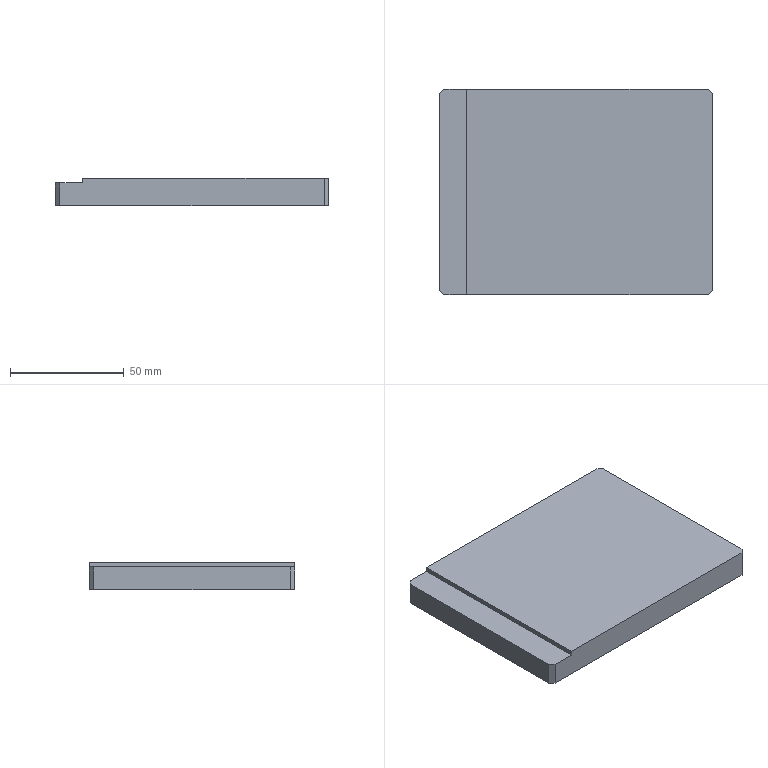Part | STEP file | 001-005-Shaft threading fixture base plate | 1 solid | 12 faces | box 120 x 90 x 12 mm | volume 127352 mm3 | plane 12
STEP:
#1=CARTESIAN_POINT('',(0.,0.,0.));
#2=DIRECTION('',(0.,0.,1.));
#3=DIRECTION('',(1.,0.,0.));
#4=AXIS2_PLACEMENT_3D('',#1,#2,#3);
#5=CARTESIAN_POINT('',(60.,-43.,12.));
#6=VERTEX_POINT('',#5);
#7=CARTESIAN_POINT('',(60.,43.,12.));
#8=VERTEX_POINT('',#7);
#9=CARTESIAN_POINT('',(60.,45.,12.));
#10=DIRECTION('',(0.,1.,0.));
#11=VECTOR('',#10,1.);
#12=LINE('',#9,#11);
#13=CARTESIAN_POINT('',(60.,45.,12.));
#14=DIRECTION('',(-1.,0.,0.));
#15=DIRECTION('',(0.,-1.,0.));
#16=AXIS2_PLACEMENT_3D('',#13,#14,#15);
#17=PLANE('',#16);
#18=CARTESIAN_POINT('',(0.,0.));
#19=DIRECTION('',(-1.,0.));
#20=VECTOR('',#19,1.);
#21=LINE('',#18,#20);
#22=(GEOMETRIC_REPRESENTATION_CONTEXT(2)PARAMETRIC_REPRESENTATION_CONTEXT()REPRESENTATION_CONTEXT('',''));
#23=DEFINITIONAL_REPRESENTATION('',(#21),#22);
#24=PCURVE('',#17,#23);
#25=CARTESIAN_POINT('',(0.,0.,12.));
#26=DIRECTION('',(0.,0.,1.));
#27=DIRECTION('',(1.,0.,0.));
#28=AXIS2_PLACEMENT_3D('',#25,#26,#27);
#29=PLANE('',#28);
#30=CARTESIAN_POINT('',(60.,45.));
#31=DIRECTION('',(0.,1.));
#32=VECTOR('',#31,1.);
#33=LINE('',#30,#32);
#34=(GEOMETRIC_REPRESENTATION_CONTEXT(2)PARAMETRIC_REPRESENTATION_CONTEXT()REPRESENTATION_CONTEXT('',''));
#35=DEFINITIONAL_REPRESENTATION('',(#33),#34);
#36=PCURVE('',#29,#35);
#37=SURFACE_CURVE('',#12,(#24,#36),.PCURVE_S1.);
#38=EDGE_CURVE('',#6,#8,#37,.T.);
#39=ORIENTED_EDGE('',*,*,#38,.F.);
#40=CARTESIAN_POINT('',(60.,-43.,0.));
#41=VERTEX_POINT('',#40);
#42=CARTESIAN_POINT('',(60.,-43.,12.));
#43=DIRECTION('',(0.,0.,-1.));
#44=VECTOR('',#43,1.);
#45=LINE('',#42,#44);
#46=CARTESIAN_POINT('',(88.,0.));
#47=DIRECTION('',(0.,-1.));
#48=VECTOR('',#47,1.);
#49=LINE('',#46,#48);
#50=(GEOMETRIC_REPRESENTATION_CONTEXT(2)PARAMETRIC_REPRESENTATION_CONTEXT()REPRESENTATION_CONTEXT('',''));
#51=DEFINITIONAL_REPRESENTATION('',(#49),#50);
#52=PCURVE('',#17,#51);
#53=CARTESIAN_POINT('',(60.,-43.,12.));
#54=DIRECTION('',(-0.7071,0.7071,0.));
#55=DIRECTION('',(0.,0.,-1.));
#56=AXIS2_PLACEMENT_3D('',#53,#54,#55);
#57=PLANE('',#56);
#58=CARTESIAN_POINT('',(0.,0.));
#59=DIRECTION('',(1.,0.));
#60=VECTOR('',#59,1.);
#61=LINE('',#58,#60);
#62=(GEOMETRIC_REPRESENTATION_CONTEXT(2)PARAMETRIC_REPRESENTATION_CONTEXT()REPRESENTATION_CONTEXT('',''));
#63=DEFINITIONAL_REPRESENTATION('',(#61),#62);
#64=PCURVE('',#57,#63);
#65=SURFACE_CURVE('',#45,(#52,#64),.PCURVE_S1.);
#66=EDGE_CURVE('',#6,#41,#65,.T.);
#67=ORIENTED_EDGE('',*,*,#66,.T.);
#68=CARTESIAN_POINT('',(60.,43.,0.));
#69=VERTEX_POINT('',#68);
#70=CARTESIAN_POINT('',(60.,45.,0.));
#71=DIRECTION('',(0.,1.,0.));
#72=VECTOR('',#71,1.);
#73=LINE('',#70,#72);
#74=CARTESIAN_POINT('',(0.,-12.));
#75=DIRECTION('',(-1.,0.));
#76=VECTOR('',#75,1.);
#77=LINE('',#74,#76);
#78=(GEOMETRIC_REPRESENTATION_CONTEXT(2)PARAMETRIC_REPRESENTATION_CONTEXT()REPRESENTATION_CONTEXT('',''));
#79=DEFINITIONAL_REPRESENTATION('',(#77),#78);
#80=PCURVE('',#17,#79);
#81=CARTESIAN_POINT('',(0.,0.,0.));
#82=DIRECTION('',(0.,0.,1.));
#83=DIRECTION('',(1.,0.,0.));
#84=AXIS2_PLACEMENT_3D('',#81,#82,#83);
#85=PLANE('',#84);
#86=CARTESIAN_POINT('',(60.,45.));
#87=DIRECTION('',(0.,1.));
#88=VECTOR('',#87,1.);
#89=LINE('',#86,#88);
#90=(GEOMETRIC_REPRESENTATION_CONTEXT(2)PARAMETRIC_REPRESENTATION_CONTEXT()REPRESENTATION_CONTEXT('',''));
#91=DEFINITIONAL_REPRESENTATION('',(#89),#90);
#92=PCURVE('',#85,#91);
#93=SURFACE_CURVE('',#73,(#80,#92),.PCURVE_S1.);
#94=EDGE_CURVE('',#41,#69,#93,.T.);
#95=ORIENTED_EDGE('',*,*,#94,.T.);
#96=CARTESIAN_POINT('',(60.,43.,12.));
#97=DIRECTION('',(0.,0.,1.));
#98=VECTOR('',#97,1.);
#99=LINE('',#96,#98);
#100=CARTESIAN_POINT('',(2.,0.));
#101=DIRECTION('',(0.,1.));
#102=VECTOR('',#101,1.);
#103=LINE('',#100,#102);
#104=(GEOMETRIC_REPRESENTATION_CONTEXT(2)PARAMETRIC_REPRESENTATION_CONTEXT()REPRESENTATION_CONTEXT('',''));
#105=DEFINITIONAL_REPRESENTATION('',(#103),#104);
#106=PCURVE('',#17,#105);
#107=CARTESIAN_POINT('',(58.,45.,12.));
#108=DIRECTION('',(-0.7071,-0.7071,0.));
#109=DIRECTION('',(0.,0.,-1.));
#110=AXIS2_PLACEMENT_3D('',#107,#108,#109);
#111=PLANE('',#110);
#112=CARTESIAN_POINT('',(0.,2.828));
#113=DIRECTION('',(-1.,0.));
#114=VECTOR('',#113,1.);
#115=LINE('',#112,#114);
#116=(GEOMETRIC_REPRESENTATION_CONTEXT(2)PARAMETRIC_REPRESENTATION_CONTEXT()REPRESENTATION_CONTEXT('',''));
#117=DEFINITIONAL_REPRESENTATION('',(#115),#116);
#118=PCURVE('',#111,#117);
#119=SURFACE_CURVE('',#99,(#106,#118),.PCURVE_S1.);
#120=EDGE_CURVE('',#69,#8,#119,.T.);
#121=ORIENTED_EDGE('',*,*,#120,.T.);
#122=EDGE_LOOP('',(#39,#67,#95,#121));
#123=FACE_BOUND('',#122,.T.);
#124=ADVANCED_FACE('',(#123),#17,.F.);
#125=CARTESIAN_POINT('',(-58.,45.,10.));
#126=VERTEX_POINT('',#125);
#127=CARTESIAN_POINT('',(-48.,45.,10.));
#128=VERTEX_POINT('',#127);
#129=CARTESIAN_POINT('',(-48.,45.,10.));
#130=DIRECTION('',(1.,0.,0.));
#131=VECTOR('',#130,1.);
#132=LINE('',#129,#131);
#133=CARTESIAN_POINT('',(-60.,45.,12.));
#134=DIRECTION('',(0.,-1.,0.));
#135=DIRECTION('',(0.,0.,-1.));
#136=AXIS2_PLACEMENT_3D('',#133,#134,#135);
#137=PLANE('',#136);
#138=CARTESIAN_POINT('',(2.,12.));
#139=DIRECTION('',(0.,1.));
#140=VECTOR('',#139,1.);
#141=LINE('',#138,#140);
#142=(GEOMETRIC_REPRESENTATION_CONTEXT(2)PARAMETRIC_REPRESENTATION_CONTEXT()REPRESENTATION_CONTEXT('',''));
#143=DEFINITIONAL_REPRESENTATION('',(#141),#142);
#144=PCURVE('',#137,#143);
#145=CARTESIAN_POINT('',(-48.,45.,10.));
#146=DIRECTION('',(0.,0.,-1.));
#147=DIRECTION('',(-1.,0.,0.));
#148=AXIS2_PLACEMENT_3D('',#145,#146,#147);
#149=PLANE('',#148);
#150=CARTESIAN_POINT('',(0.,0.));
#151=DIRECTION('',(-1.,0.));
#152=VECTOR('',#151,1.);
#153=LINE('',#150,#152);
#154=(GEOMETRIC_REPRESENTATION_CONTEXT(2)PARAMETRIC_REPRESENTATION_CONTEXT()REPRESENTATION_CONTEXT('',''));
#155=DEFINITIONAL_REPRESENTATION('',(#153),#154);
#156=PCURVE('',#149,#155);
#157=SURFACE_CURVE('',#132,(#144,#156),.PCURVE_S1.);
#158=EDGE_CURVE('',#126,#128,#157,.T.);
#159=ORIENTED_EDGE('',*,*,#158,.T.);
#160=CARTESIAN_POINT('',(-48.,45.,12.));
#161=VERTEX_POINT('',#160);
#162=CARTESIAN_POINT('',(-48.,45.,12.));
#163=DIRECTION('',(0.,0.,1.));
#164=VECTOR('',#163,1.);
#165=LINE('',#162,#164);
#166=CARTESIAN_POINT('',(0.,12.));
#167=DIRECTION('',(-1.,0.));
#168=VECTOR('',#167,1.);
#169=LINE('',#166,#168);
#170=(GEOMETRIC_REPRESENTATION_CONTEXT(2)PARAMETRIC_REPRESENTATION_CONTEXT()REPRESENTATION_CONTEXT('',''));
#171=DEFINITIONAL_REPRESENTATION('',(#169),#170);
#172=PCURVE('',#137,#171);
#173=CARTESIAN_POINT('',(-48.,45.,12.));
#174=DIRECTION('',(1.,0.,0.));
#175=DIRECTION('',(0.,1.,0.));
#176=AXIS2_PLACEMENT_3D('',#173,#174,#175);
#177=PLANE('',#176);
#178=CARTESIAN_POINT('',(0.,0.));
#179=DIRECTION('',(0.,1.));
#180=VECTOR('',#179,1.);
#181=LINE('',#178,#180);
#182=(GEOMETRIC_REPRESENTATION_CONTEXT(2)PARAMETRIC_REPRESENTATION_CONTEXT()REPRESENTATION_CONTEXT('',''));
#183=DEFINITIONAL_REPRESENTATION('',(#181),#182);
#184=PCURVE('',#177,#183);
#185=SURFACE_CURVE('',#165,(#172,#184),.PCURVE_S1.);
#186=EDGE_CURVE('',#128,#161,#185,.T.);
#187=ORIENTED_EDGE('',*,*,#186,.T.);
#188=CARTESIAN_POINT('',(58.,45.,12.));
#189=VERTEX_POINT('',#188);
#190=CARTESIAN_POINT('',(-60.,45.,12.));
#191=DIRECTION('',(-1.,0.,0.));
#192=VECTOR('',#191,1.);
#193=LINE('',#190,#192);
#194=CARTESIAN_POINT('',(0.,0.));
#195=DIRECTION('',(0.,-1.));
#196=VECTOR('',#195,1.);
#197=LINE('',#194,#196);
#198=(GEOMETRIC_REPRESENTATION_CONTEXT(2)PARAMETRIC_REPRESENTATION_CONTEXT()REPRESENTATION_CONTEXT('',''));
#199=DEFINITIONAL_REPRESENTATION('',(#197),#198);
#200=PCURVE('',#137,#199);
#201=CARTESIAN_POINT('',(-60.,45.));
#202=DIRECTION('',(-1.,0.));
#203=VECTOR('',#202,1.);
#204=LINE('',#201,#203);
#205=(GEOMETRIC_REPRESENTATION_CONTEXT(2)PARAMETRIC_REPRESENTATION_CONTEXT()REPRESENTATION_CONTEXT('',''));
#206=DEFINITIONAL_REPRESENTATION('',(#204),#205);
#207=PCURVE('',#29,#206);
#208=SURFACE_CURVE('',#193,(#200,#207),.PCURVE_S1.);
#209=EDGE_CURVE('',#189,#161,#208,.T.);
#210=ORIENTED_EDGE('',*,*,#209,.F.);
#211=CARTESIAN_POINT('',(58.,45.,0.));
#212=VERTEX_POINT('',#211);
#213=CARTESIAN_POINT('',(58.,45.,12.));
#214=DIRECTION('',(0.,0.,-1.));
#215=VECTOR('',#214,1.);
#216=LINE('',#213,#215);
#217=CARTESIAN_POINT('',(0.,118.));
#218=DIRECTION('',(1.,0.));
#219=VECTOR('',#218,1.);
#220=LINE('',#217,#219);
#221=(GEOMETRIC_REPRESENTATION_CONTEXT(2)PARAMETRIC_REPRESENTATION_CONTEXT()REPRESENTATION_CONTEXT('',''));
#222=DEFINITIONAL_REPRESENTATION('',(#220),#221);
#223=PCURVE('',#137,#222);
#224=CARTESIAN_POINT('',(0.,0.));
#225=DIRECTION('',(1.,0.));
#226=VECTOR('',#225,1.);
#227=LINE('',#224,#226);
#228=(GEOMETRIC_REPRESENTATION_CONTEXT(2)PARAMETRIC_REPRESENTATION_CONTEXT()REPRESENTATION_CONTEXT('',''));
#229=DEFINITIONAL_REPRESENTATION('',(#227),#228);
#230=PCURVE('',#111,#229);
#231=SURFACE_CURVE('',#216,(#223,#230),.PCURVE_S1.);
#232=EDGE_CURVE('',#189,#212,#231,.T.);
#233=ORIENTED_EDGE('',*,*,#232,.T.);
#234=CARTESIAN_POINT('',(-58.,45.,0.));
#235=VERTEX_POINT('',#234);
#236=CARTESIAN_POINT('',(-60.,45.,0.));
#237=DIRECTION('',(-1.,0.,0.));
#238=VECTOR('',#237,1.);
#239=LINE('',#236,#238);
#240=CARTESIAN_POINT('',(12.,0.));
#241=DIRECTION('',(0.,-1.));
#242=VECTOR('',#241,1.);
#243=LINE('',#240,#242);
#244=(GEOMETRIC_REPRESENTATION_CONTEXT(2)PARAMETRIC_REPRESENTATION_CONTEXT()REPRESENTATION_CONTEXT('',''));
#245=DEFINITIONAL_REPRESENTATION('',(#243),#244);
#246=PCURVE('',#137,#245);
#247=CARTESIAN_POINT('',(-60.,45.));
#248=DIRECTION('',(-1.,0.));
#249=VECTOR('',#248,1.);
#250=LINE('',#247,#249);
#251=(GEOMETRIC_REPRESENTATION_CONTEXT(2)PARAMETRIC_REPRESENTATION_CONTEXT()REPRESENTATION_CONTEXT('',''));
#252=DEFINITIONAL_REPRESENTATION('',(#250),#251);
#253=PCURVE('',#85,#252);
#254=SURFACE_CURVE('',#239,(#246,#253),.PCURVE_S1.);
#255=EDGE_CURVE('',#212,#235,#254,.T.);
#256=ORIENTED_EDGE('',*,*,#255,.T.);
#257=CARTESIAN_POINT('',(-58.,45.,12.));
#258=DIRECTION('',(0.,0.,1.));
#259=VECTOR('',#258,1.);
#260=LINE('',#257,#259);
#261=CARTESIAN_POINT('',(0.,2.));
#262=DIRECTION('',(-1.,0.));
#263=VECTOR('',#262,1.);
#264=LINE('',#261,#263);
#265=(GEOMETRIC_REPRESENTATION_CONTEXT(2)PARAMETRIC_REPRESENTATION_CONTEXT()REPRESENTATION_CONTEXT('',''));
#266=DEFINITIONAL_REPRESENTATION('',(#264),#265);
#267=PCURVE('',#137,#266);
#268=CARTESIAN_POINT('',(-60.,43.,12.));
#269=DIRECTION('',(0.7071,-0.7071,0.));
#270=DIRECTION('',(0.,0.,-1.));
#271=AXIS2_PLACEMENT_3D('',#268,#269,#270);
#272=PLANE('',#271);
#273=CARTESIAN_POINT('',(0.,2.828));
#274=DIRECTION('',(-1.,0.));
#275=VECTOR('',#274,1.);
#276=LINE('',#273,#275);
#277=(GEOMETRIC_REPRESENTATION_CONTEXT(2)PARAMETRIC_REPRESENTATION_CONTEXT()REPRESENTATION_CONTEXT('',''));
#278=DEFINITIONAL_REPRESENTATION('',(#276),#277);
#279=PCURVE('',#272,#278);
#280=SURFACE_CURVE('',#260,(#267,#279),.PCURVE_S1.);
#281=EDGE_CURVE('',#235,#126,#280,.T.);
#282=ORIENTED_EDGE('',*,*,#281,.T.);
#283=EDGE_LOOP('',(#159,#187,#210,#233,#256,#282));
#284=FACE_BOUND('',#283,.T.);
#285=ADVANCED_FACE('',(#284),#137,.F.);
#286=CARTESIAN_POINT('',(-60.,-43.,0.));
#287=VERTEX_POINT('',#286);
#288=CARTESIAN_POINT('',(-60.,-43.,10.));
#289=VERTEX_POINT('',#288);
#290=CARTESIAN_POINT('',(-60.,-43.,12.));
#291=DIRECTION('',(0.,0.,1.));
#292=VECTOR('',#291,1.);
#293=LINE('',#290,#292);
#294=CARTESIAN_POINT('',(-60.,45.,12.));
#295=DIRECTION('',(1.,0.,0.));
#296=DIRECTION('',(0.,1.,0.));
#297=AXIS2_PLACEMENT_3D('',#294,#295,#296);
#298=PLANE('',#297);
#299=CARTESIAN_POINT('',(-88.,0.));
#300=DIRECTION('',(0.,1.));
#301=VECTOR('',#300,1.);
#302=LINE('',#299,#301);
#303=(GEOMETRIC_REPRESENTATION_CONTEXT(2)PARAMETRIC_REPRESENTATION_CONTEXT()REPRESENTATION_CONTEXT('',''));
#304=DEFINITIONAL_REPRESENTATION('',(#302),#303);
#305=PCURVE('',#298,#304);
#306=CARTESIAN_POINT('',(-58.,-45.,12.));
#307=DIRECTION('',(0.7071,0.7071,0.));
#308=DIRECTION('',(0.,0.,-1.));
#309=AXIS2_PLACEMENT_3D('',#306,#307,#308);
#310=PLANE('',#309);
#311=CARTESIAN_POINT('',(0.,2.828));
#312=DIRECTION('',(-1.,0.));
#313=VECTOR('',#312,1.);
#314=LINE('',#311,#313);
#315=(GEOMETRIC_REPRESENTATION_CONTEXT(2)PARAMETRIC_REPRESENTATION_CONTEXT()REPRESENTATION_CONTEXT('',''));
#316=DEFINITIONAL_REPRESENTATION('',(#314),#315);
#317=PCURVE('',#310,#316);
#318=SURFACE_CURVE('',#293,(#305,#317),.PCURVE_S1.);
#319=EDGE_CURVE('',#287,#289,#318,.T.);
#320=ORIENTED_EDGE('',*,*,#319,.T.);
#321=CARTESIAN_POINT('',(-60.,43.,10.));
#322=VERTEX_POINT('',#321);
#323=CARTESIAN_POINT('',(-60.,45.,10.));
#324=DIRECTION('',(0.,-1.,0.));
#325=VECTOR('',#324,1.);
#326=LINE('',#323,#325);
#327=CARTESIAN_POINT('',(0.,-2.));
#328=DIRECTION('',(-1.,0.));
#329=VECTOR('',#328,1.);
#330=LINE('',#327,#329);
#331=(GEOMETRIC_REPRESENTATION_CONTEXT(2)PARAMETRIC_REPRESENTATION_CONTEXT()REPRESENTATION_CONTEXT('',''));
#332=DEFINITIONAL_REPRESENTATION('',(#330),#331);
#333=PCURVE('',#298,#332);
#334=CARTESIAN_POINT('',(12.,0.));
#335=DIRECTION('',(0.,-1.));
#336=VECTOR('',#335,1.);
#337=LINE('',#334,#336);
#338=(GEOMETRIC_REPRESENTATION_CONTEXT(2)PARAMETRIC_REPRESENTATION_CONTEXT()REPRESENTATION_CONTEXT('',''));
#339=DEFINITIONAL_REPRESENTATION('',(#337),#338);
#340=PCURVE('',#149,#339);
#341=SURFACE_CURVE('',#326,(#333,#340),.PCURVE_S1.);
#342=EDGE_CURVE('',#322,#289,#341,.T.);
#343=ORIENTED_EDGE('',*,*,#342,.F.);
#344=CARTESIAN_POINT('',(-60.,43.,0.));
#345=VERTEX_POINT('',#344);
#346=CARTESIAN_POINT('',(-60.,43.,12.));
#347=DIRECTION('',(0.,0.,-1.));
#348=VECTOR('',#347,1.);
#349=LINE('',#346,#348);
#350=CARTESIAN_POINT('',(-2.,0.));
#351=DIRECTION('',(0.,-1.));
#352=VECTOR('',#351,1.);
#353=LINE('',#350,#352);
#354=(GEOMETRIC_REPRESENTATION_CONTEXT(2)PARAMETRIC_REPRESENTATION_CONTEXT()REPRESENTATION_CONTEXT('',''));
#355=DEFINITIONAL_REPRESENTATION('',(#353),#354);
#356=PCURVE('',#298,#355);
#357=CARTESIAN_POINT('',(0.,0.));
#358=DIRECTION('',(1.,0.));
#359=VECTOR('',#358,1.);
#360=LINE('',#357,#359);
#361=(GEOMETRIC_REPRESENTATION_CONTEXT(2)PARAMETRIC_REPRESENTATION_CONTEXT()REPRESENTATION_CONTEXT('',''));
#362=DEFINITIONAL_REPRESENTATION('',(#360),#361);
#363=PCURVE('',#272,#362);
#364=SURFACE_CURVE('',#349,(#356,#363),.PCURVE_S1.);
#365=EDGE_CURVE('',#322,#345,#364,.T.);
#366=ORIENTED_EDGE('',*,*,#365,.T.);
#367=CARTESIAN_POINT('',(-60.,45.,0.));
#368=DIRECTION('',(0.,-1.,0.));
#369=VECTOR('',#368,1.);
#370=LINE('',#367,#369);
#371=CARTESIAN_POINT('',(0.,-12.));
#372=DIRECTION('',(-1.,0.));
#373=VECTOR('',#372,1.);
#374=LINE('',#371,#373);
#375=(GEOMETRIC_REPRESENTATION_CONTEXT(2)PARAMETRIC_REPRESENTATION_CONTEXT()REPRESENTATION_CONTEXT('',''));
#376=DEFINITIONAL_REPRESENTATION('',(#374),#375);
#377=PCURVE('',#298,#376);
#378=CARTESIAN_POINT('',(-60.,45.));
#379=DIRECTION('',(0.,-1.));
#380=VECTOR('',#379,1.);
#381=LINE('',#378,#380);
#382=(GEOMETRIC_REPRESENTATION_CONTEXT(2)PARAMETRIC_REPRESENTATION_CONTEXT()REPRESENTATION_CONTEXT('',''));
#383=DEFINITIONAL_REPRESENTATION('',(#381),#382);
#384=PCURVE('',#85,#383);
#385=SURFACE_CURVE('',#370,(#377,#384),.PCURVE_S1.);
#386=EDGE_CURVE('',#345,#287,#385,.T.);
#387=ORIENTED_EDGE('',*,*,#386,.T.);
#388=EDGE_LOOP('',(#320,#343,#366,#387));
#389=FACE_BOUND('',#388,.T.);
#390=ADVANCED_FACE('',(#389),#298,.F.);
#391=CARTESIAN_POINT('',(-48.,-45.,12.));
#392=VERTEX_POINT('',#391);
#393=CARTESIAN_POINT('',(58.,-45.,12.));
#394=VERTEX_POINT('',#393);
#395=CARTESIAN_POINT('',(-60.,-45.,12.));
#396=DIRECTION('',(1.,0.,0.));
#397=VECTOR('',#396,1.);
#398=LINE('',#395,#397);
#399=CARTESIAN_POINT('',(-60.,-45.,12.));
#400=DIRECTION('',(0.,1.,0.));
#401=DIRECTION('',(-1.,0.,0.));
#402=AXIS2_PLACEMENT_3D('',#399,#400,#401);
#403=PLANE('',#402);
#404=CARTESIAN_POINT('',(0.,0.));
#405=DIRECTION('',(-1.,0.));
#406=VECTOR('',#405,1.);
#407=LINE('',#404,#406);
#408=(GEOMETRIC_REPRESENTATION_CONTEXT(2)PARAMETRIC_REPRESENTATION_CONTEXT()REPRESENTATION_CONTEXT('',''));
#409=DEFINITIONAL_REPRESENTATION('',(#407),#408);
#410=PCURVE('',#403,#409);
#411=CARTESIAN_POINT('',(-60.,-45.));
#412=DIRECTION('',(1.,0.));
#413=VECTOR('',#412,1.);
#414=LINE('',#411,#413);
#415=(GEOMETRIC_REPRESENTATION_CONTEXT(2)PARAMETRIC_REPRESENTATION_CONTEXT()REPRESENTATION_CONTEXT('',''));
#416=DEFINITIONAL_REPRESENTATION('',(#414),#415);
#417=PCURVE('',#29,#416);
#418=SURFACE_CURVE('',#398,(#410,#417),.PCURVE_S1.);
#419=EDGE_CURVE('',#392,#394,#418,.T.);
#420=ORIENTED_EDGE('',*,*,#419,.F.);
#421=CARTESIAN_POINT('',(-48.,-45.,10.));
#422=VERTEX_POINT('',#421);
#423=CARTESIAN_POINT('',(-48.,-45.,12.));
#424=DIRECTION('',(0.,0.,1.));
#425=VECTOR('',#424,1.);
#426=LINE('',#423,#425);
#427=CARTESIAN_POINT('',(-12.,0.));
#428=DIRECTION('',(0.,1.));
#429=VECTOR('',#428,1.);
#430=LINE('',#427,#429);
#431=(GEOMETRIC_REPRESENTATION_CONTEXT(2)PARAMETRIC_REPRESENTATION_CONTEXT()REPRESENTATION_CONTEXT('',''));
#432=DEFINITIONAL_REPRESENTATION('',(#430),#431);
#433=PCURVE('',#403,#432);
#434=CARTESIAN_POINT('',(-90.,0.));
#435=DIRECTION('',(0.,1.));
#436=VECTOR('',#435,1.);
#437=LINE('',#434,#436);
#438=(GEOMETRIC_REPRESENTATION_CONTEXT(2)PARAMETRIC_REPRESENTATION_CONTEXT()REPRESENTATION_CONTEXT('',''));
#439=DEFINITIONAL_REPRESENTATION('',(#437),#438);
#440=PCURVE('',#177,#439);
#441=SURFACE_CURVE('',#426,(#433,#440),.PCURVE_S1.);
#442=EDGE_CURVE('',#422,#392,#441,.T.);
#443=ORIENTED_EDGE('',*,*,#442,.F.);
#444=CARTESIAN_POINT('',(-58.,-45.,10.));
#445=VERTEX_POINT('',#444);
#446=CARTESIAN_POINT('',(-48.,-45.,10.));
#447=DIRECTION('',(1.,0.,0.));
#448=VECTOR('',#447,1.);
#449=LINE('',#446,#448);
#450=CARTESIAN_POINT('',(-12.,-2.));
#451=DIRECTION('',(-1.,0.));
#452=VECTOR('',#451,1.);
#453=LINE('',#450,#452);
#454=(GEOMETRIC_REPRESENTATION_CONTEXT(2)PARAMETRIC_REPRESENTATION_CONTEXT()REPRESENTATION_CONTEXT('',''));
#455=DEFINITIONAL_REPRESENTATION('',(#453),#454);
#456=PCURVE('',#403,#455);
#457=CARTESIAN_POINT('',(0.,-90.));
#458=DIRECTION('',(-1.,0.));
#459=VECTOR('',#458,1.);
#460=LINE('',#457,#459);
#461=(GEOMETRIC_REPRESENTATION_CONTEXT(2)PARAMETRIC_REPRESENTATION_CONTEXT()REPRESENTATION_CONTEXT('',''));
#462=DEFINITIONAL_REPRESENTATION('',(#460),#461);
#463=PCURVE('',#149,#462);
#464=SURFACE_CURVE('',#449,(#456,#463),.PCURVE_S1.);
#465=EDGE_CURVE('',#445,#422,#464,.T.);
#466=ORIENTED_EDGE('',*,*,#465,.F.);
#467=CARTESIAN_POINT('',(-58.,-45.,0.));
#468=VERTEX_POINT('',#467);
#469=CARTESIAN_POINT('',(-58.,-45.,12.));
#470=DIRECTION('',(0.,0.,-1.));
#471=VECTOR('',#470,1.);
#472=LINE('',#469,#471);
#473=CARTESIAN_POINT('',(-2.,0.));
#474=DIRECTION('',(0.,-1.));
#475=VECTOR('',#474,1.);
#476=LINE('',#473,#475);
#477=(GEOMETRIC_REPRESENTATION_CONTEXT(2)PARAMETRIC_REPRESENTATION_CONTEXT()REPRESENTATION_CONTEXT('',''));
#478=DEFINITIONAL_REPRESENTATION('',(#476),#477);
#479=PCURVE('',#403,#478);
#480=CARTESIAN_POINT('',(0.,0.));
#481=DIRECTION('',(1.,0.));
#482=VECTOR('',#481,1.);
#483=LINE('',#480,#482);
#484=(GEOMETRIC_REPRESENTATION_CONTEXT(2)PARAMETRIC_REPRESENTATION_CONTEXT()REPRESENTATION_CONTEXT('',''));
#485=DEFINITIONAL_REPRESENTATION('',(#483),#484);
#486=PCURVE('',#310,#485);
#487=SURFACE_CURVE('',#472,(#479,#486),.PCURVE_S1.);
#488=EDGE_CURVE('',#445,#468,#487,.T.);
#489=ORIENTED_EDGE('',*,*,#488,.T.);
#490=CARTESIAN_POINT('',(58.,-45.,0.));
#491=VERTEX_POINT('',#490);
#492=CARTESIAN_POINT('',(-60.,-45.,0.));
#493=DIRECTION('',(1.,0.,0.));
#494=VECTOR('',#493,1.);
#495=LINE('',#492,#494);
#496=CARTESIAN_POINT('',(0.,-12.));
#497=DIRECTION('',(-1.,0.));
#498=VECTOR('',#497,1.);
#499=LINE('',#496,#498);
#500=(GEOMETRIC_REPRESENTATION_CONTEXT(2)PARAMETRIC_REPRESENTATION_CONTEXT()REPRESENTATION_CONTEXT('',''));
#501=DEFINITIONAL_REPRESENTATION('',(#499),#500);
#502=PCURVE('',#403,#501);
#503=CARTESIAN_POINT('',(-60.,-45.));
#504=DIRECTION('',(1.,0.));
#505=VECTOR('',#504,1.);
#506=LINE('',#503,#505);
#507=(GEOMETRIC_REPRESENTATION_CONTEXT(2)PARAMETRIC_REPRESENTATION_CONTEXT()REPRESENTATION_CONTEXT('',''));
#508=DEFINITIONAL_REPRESENTATION('',(#506),#507);
#509=PCURVE('',#85,#508);
#510=SURFACE_CURVE('',#495,(#502,#509),.PCURVE_S1.);
#511=EDGE_CURVE('',#468,#491,#510,.T.);
#512=ORIENTED_EDGE('',*,*,#511,.T.);
#513=CARTESIAN_POINT('',(58.,-45.,12.));
#514=DIRECTION('',(0.,0.,1.));
#515=VECTOR('',#514,1.);
#516=LINE('',#513,#515);
#517=CARTESIAN_POINT('',(-118.,0.));
#518=DIRECTION('',(0.,1.));
#519=VECTOR('',#518,1.);
#520=LINE('',#517,#519);
#521=(GEOMETRIC_REPRESENTATION_CONTEXT(2)PARAMETRIC_REPRESENTATION_CONTEXT()REPRESENTATION_CONTEXT('',''));
#522=DEFINITIONAL_REPRESENTATION('',(#520),#521);
#523=PCURVE('',#403,#522);
#524=CARTESIAN_POINT('',(0.,2.828));
#525=DIRECTION('',(-1.,0.));
#526=VECTOR('',#525,1.);
#527=LINE('',#524,#526);
#528=(GEOMETRIC_REPRESENTATION_CONTEXT(2)PARAMETRIC_REPRESENTATION_CONTEXT()REPRESENTATION_CONTEXT('',''));
#529=DEFINITIONAL_REPRESENTATION('',(#527),#528);
#530=PCURVE('',#57,#529);
#531=SURFACE_CURVE('',#516,(#523,#530),.PCURVE_S1.);
#532=EDGE_CURVE('',#491,#394,#531,.T.);
#533=ORIENTED_EDGE('',*,*,#532,.T.);
#534=EDGE_LOOP('',(#420,#443,#466,#489,#512,#533));
#535=FACE_BOUND('',#534,.T.);
#536=ADVANCED_FACE('',(#535),#403,.F.);
#537=CARTESIAN_POINT('',(-48.,45.,12.));
#538=DIRECTION('',(0.,-1.,0.));
#539=VECTOR('',#538,1.);
#540=LINE('',#537,#539);
#541=CARTESIAN_POINT('',(-48.,45.));
#542=DIRECTION('',(0.,-1.));
#543=VECTOR('',#542,1.);
#544=LINE('',#541,#543);
#545=(GEOMETRIC_REPRESENTATION_CONTEXT(2)PARAMETRIC_REPRESENTATION_CONTEXT()REPRESENTATION_CONTEXT('',''));
#546=DEFINITIONAL_REPRESENTATION('',(#544),#545);
#547=PCURVE('',#29,#546);
#548=CARTESIAN_POINT('',(0.,0.));
#549=DIRECTION('',(-1.,0.));
#550=VECTOR('',#549,1.);
#551=LINE('',#548,#550);
#552=(GEOMETRIC_REPRESENTATION_CONTEXT(2)PARAMETRIC_REPRESENTATION_CONTEXT()REPRESENTATION_CONTEXT('',''));
#553=DEFINITIONAL_REPRESENTATION('',(#551),#552);
#554=PCURVE('',#177,#553);
#555=SURFACE_CURVE('',#540,(#547,#554),.PCURVE_S1.);
#556=EDGE_CURVE('',#161,#392,#555,.T.);
#557=ORIENTED_EDGE('',*,*,#556,.T.);
#558=ORIENTED_EDGE('',*,*,#419,.T.);
#559=CARTESIAN_POINT('',(51.5,-51.5,12.));
#560=DIRECTION('',(0.7071,0.7071,0.));
#561=VECTOR('',#560,1.);
#562=LINE('',#559,#561);
#563=CARTESIAN_POINT('',(51.5,-51.5));
#564=DIRECTION('',(0.7071,0.7071));
#565=VECTOR('',#564,1.);
#566=LINE('',#563,#565);
#567=(GEOMETRIC_REPRESENTATION_CONTEXT(2)PARAMETRIC_REPRESENTATION_CONTEXT()REPRESENTATION_CONTEXT('',''));
#568=DEFINITIONAL_REPRESENTATION('',(#566),#567);
#569=PCURVE('',#29,#568);
#570=CARTESIAN_POINT('',(0.,12.021));
#571=DIRECTION('',(0.,-1.));
#572=VECTOR('',#571,1.);
#573=LINE('',#570,#572);
#574=(GEOMETRIC_REPRESENTATION_CONTEXT(2)PARAMETRIC_REPRESENTATION_CONTEXT()REPRESENTATION_CONTEXT('',''));
#575=DEFINITIONAL_REPRESENTATION('',(#573),#574);
#576=PCURVE('',#57,#575);
#577=SURFACE_CURVE('',#562,(#569,#576),.PCURVE_S1.);
#578=EDGE_CURVE('',#394,#6,#577,.T.);
#579=ORIENTED_EDGE('',*,*,#578,.T.);
#580=ORIENTED_EDGE('',*,*,#38,.T.);
#581=CARTESIAN_POINT('',(51.5,51.5,12.));
#582=DIRECTION('',(-0.7071,0.7071,0.));
#583=VECTOR('',#582,1.);
#584=LINE('',#581,#583);
#585=CARTESIAN_POINT('',(51.5,51.5));
#586=DIRECTION('',(-0.7071,0.7071));
#587=VECTOR('',#586,1.);
#588=LINE('',#585,#587);
#589=(GEOMETRIC_REPRESENTATION_CONTEXT(2)PARAMETRIC_REPRESENTATION_CONTEXT()REPRESENTATION_CONTEXT('',''));
#590=DEFINITIONAL_REPRESENTATION('',(#588),#589);
#591=PCURVE('',#29,#590);
#592=CARTESIAN_POINT('',(0.,-9.192));
#593=DIRECTION('',(0.,-1.));
#594=VECTOR('',#593,1.);
#595=LINE('',#592,#594);
#596=(GEOMETRIC_REPRESENTATION_CONTEXT(2)PARAMETRIC_REPRESENTATION_CONTEXT()REPRESENTATION_CONTEXT('',''));
#597=DEFINITIONAL_REPRESENTATION('',(#595),#596);
#598=PCURVE('',#111,#597);
#599=SURFACE_CURVE('',#584,(#591,#598),.PCURVE_S1.);
#600=EDGE_CURVE('',#8,#189,#599,.T.);
#601=ORIENTED_EDGE('',*,*,#600,.T.);
#602=ORIENTED_EDGE('',*,*,#209,.T.);
#603=EDGE_LOOP('',(#557,#558,#579,#580,#601,#602));
#604=FACE_BOUND('',#603,.T.);
#605=ADVANCED_FACE('',(#604),#29,.T.);
#606=ORIENTED_EDGE('',*,*,#94,.F.);
#607=CARTESIAN_POINT('',(60.,-43.,0.));
#608=DIRECTION('',(-0.7071,-0.7071,0.));
#609=VECTOR('',#608,1.);
#610=LINE('',#607,#609);
#611=CARTESIAN_POINT('',(60.,-43.));
#612=DIRECTION('',(-0.7071,-0.7071));
#613=VECTOR('',#612,1.);
#614=LINE('',#611,#613);
#615=(GEOMETRIC_REPRESENTATION_CONTEXT(2)PARAMETRIC_REPRESENTATION_CONTEXT()REPRESENTATION_CONTEXT('',''));
#616=DEFINITIONAL_REPRESENTATION('',(#614),#615);
#617=PCURVE('',#85,#616);
#618=CARTESIAN_POINT('',(12.,0.));
#619=DIRECTION('',(0.,1.));
#620=VECTOR('',#619,1.);
#621=LINE('',#618,#620);
#622=(GEOMETRIC_REPRESENTATION_CONTEXT(2)PARAMETRIC_REPRESENTATION_CONTEXT()REPRESENTATION_CONTEXT('',''));
#623=DEFINITIONAL_REPRESENTATION('',(#621),#622);
#624=PCURVE('',#57,#623);
#625=SURFACE_CURVE('',#610,(#617,#624),.PCURVE_S1.);
#626=EDGE_CURVE('',#41,#491,#625,.T.);
#627=ORIENTED_EDGE('',*,*,#626,.T.);
#628=ORIENTED_EDGE('',*,*,#511,.F.);
#629=CARTESIAN_POINT('',(-58.,-45.,0.));
#630=DIRECTION('',(-0.7071,0.7071,0.));
#631=VECTOR('',#630,1.);
#632=LINE('',#629,#631);
#633=CARTESIAN_POINT('',(-58.,-45.));
#634=DIRECTION('',(-0.7071,0.7071));
#635=VECTOR('',#634,1.);
#636=LINE('',#633,#635);
#637=(GEOMETRIC_REPRESENTATION_CONTEXT(2)PARAMETRIC_REPRESENTATION_CONTEXT()REPRESENTATION_CONTEXT('',''));
#638=DEFINITIONAL_REPRESENTATION('',(#636),#637);
#639=PCURVE('',#85,#638);
#640=CARTESIAN_POINT('',(12.,0.));
#641=DIRECTION('',(0.,1.));
#642=VECTOR('',#641,1.);
#643=LINE('',#640,#642);
#644=(GEOMETRIC_REPRESENTATION_CONTEXT(2)PARAMETRIC_REPRESENTATION_CONTEXT()REPRESENTATION_CONTEXT('',''));
#645=DEFINITIONAL_REPRESENTATION('',(#643),#644);
#646=PCURVE('',#310,#645);
#647=SURFACE_CURVE('',#632,(#639,#646),.PCURVE_S1.);
#648=EDGE_CURVE('',#468,#287,#647,.T.);
#649=ORIENTED_EDGE('',*,*,#648,.T.);
#650=ORIENTED_EDGE('',*,*,#386,.F.);
#651=CARTESIAN_POINT('',(-60.,43.,0.));
#652=DIRECTION('',(0.7071,0.7071,0.));
#653=VECTOR('',#652,1.);
#654=LINE('',#651,#653);
#655=CARTESIAN_POINT('',(-60.,43.));
#656=DIRECTION('',(0.7071,0.7071));
#657=VECTOR('',#656,1.);
#658=LINE('',#655,#657);
#659=(GEOMETRIC_REPRESENTATION_CONTEXT(2)PARAMETRIC_REPRESENTATION_CONTEXT()REPRESENTATION_CONTEXT('',''));
#660=DEFINITIONAL_REPRESENTATION('',(#658),#659);
#661=PCURVE('',#85,#660);
#662=CARTESIAN_POINT('',(12.,0.));
#663=DIRECTION('',(0.,1.));
#664=VECTOR('',#663,1.);
#665=LINE('',#662,#664);
#666=(GEOMETRIC_REPRESENTATION_CONTEXT(2)PARAMETRIC_REPRESENTATION_CONTEXT()REPRESENTATION_CONTEXT('',''));
#667=DEFINITIONAL_REPRESENTATION('',(#665),#666);
#668=PCURVE('',#272,#667);
#669=SURFACE_CURVE('',#654,(#661,#668),.PCURVE_S1.);
#670=EDGE_CURVE('',#345,#235,#669,.T.);
#671=ORIENTED_EDGE('',*,*,#670,.T.);
#672=ORIENTED_EDGE('',*,*,#255,.F.);
#673=CARTESIAN_POINT('',(58.,45.,0.));
#674=DIRECTION('',(0.7071,-0.7071,0.));
#675=VECTOR('',#674,1.);
#676=LINE('',#673,#675);
#677=CARTESIAN_POINT('',(58.,45.));
#678=DIRECTION('',(0.7071,-0.7071));
#679=VECTOR('',#678,1.);
#680=LINE('',#677,#679);
#681=(GEOMETRIC_REPRESENTATION_CONTEXT(2)PARAMETRIC_REPRESENTATION_CONTEXT()REPRESENTATION_CONTEXT('',''));
#682=DEFINITIONAL_REPRESENTATION('',(#680),#681);
#683=PCURVE('',#85,#682);
#684=CARTESIAN_POINT('',(12.,0.));
#685=DIRECTION('',(0.,1.));
#686=VECTOR('',#685,1.);
#687=LINE('',#684,#686);
#688=(GEOMETRIC_REPRESENTATION_CONTEXT(2)PARAMETRIC_REPRESENTATION_CONTEXT()REPRESENTATION_CONTEXT('',''));
#689=DEFINITIONAL_REPRESENTATION('',(#687),#688);
#690=PCURVE('',#111,#689);
#691=SURFACE_CURVE('',#676,(#683,#690),.PCURVE_S1.);
#692=EDGE_CURVE('',#212,#69,#691,.T.);
#693=ORIENTED_EDGE('',*,*,#692,.T.);
#694=EDGE_LOOP('',(#606,#627,#628,#649,#650,#671,#672,#693));
#695=FACE_BOUND('',#694,.T.);
#696=ADVANCED_FACE('',(#695),#85,.F.);
#697=ORIENTED_EDGE('',*,*,#578,.F.);
#698=ORIENTED_EDGE('',*,*,#532,.F.);
#699=ORIENTED_EDGE('',*,*,#626,.F.);
#700=ORIENTED_EDGE('',*,*,#66,.F.);
#701=EDGE_LOOP('',(#697,#698,#699,#700));
#702=FACE_BOUND('',#701,.T.);
#703=ADVANCED_FACE('',(#702),#57,.F.);
#704=CARTESIAN_POINT('',(-58.,-45.,10.));
#705=DIRECTION('',(0.7071,-0.7071,0.));
#706=VECTOR('',#705,1.);
#707=LINE('',#704,#706);
#708=CARTESIAN_POINT('',(2.,0.));
#709=DIRECTION('',(0.,-1.));
#710=VECTOR('',#709,1.);
#711=LINE('',#708,#710);
#712=(GEOMETRIC_REPRESENTATION_CONTEXT(2)PARAMETRIC_REPRESENTATION_CONTEXT()REPRESENTATION_CONTEXT('',''));
#713=DEFINITIONAL_REPRESENTATION('',(#711),#712);
#714=PCURVE('',#310,#713);
#715=CARTESIAN_POINT('',(10.,-90.));
#716=DIRECTION('',(-0.7071,-0.7071));
#717=VECTOR('',#716,1.);
#718=LINE('',#715,#717);
#719=(GEOMETRIC_REPRESENTATION_CONTEXT(2)PARAMETRIC_REPRESENTATION_CONTEXT()REPRESENTATION_CONTEXT('',''));
#720=DEFINITIONAL_REPRESENTATION('',(#718),#719);
#721=PCURVE('',#149,#720);
#722=SURFACE_CURVE('',#707,(#714,#721),.PCURVE_S1.);
#723=EDGE_CURVE('',#289,#445,#722,.T.);
#724=ORIENTED_EDGE('',*,*,#723,.F.);
#725=ORIENTED_EDGE('',*,*,#319,.F.);
#726=ORIENTED_EDGE('',*,*,#648,.F.);
#727=ORIENTED_EDGE('',*,*,#488,.F.);
#728=EDGE_LOOP('',(#724,#725,#726,#727));
#729=FACE_BOUND('',#728,.T.);
#730=ADVANCED_FACE('',(#729),#310,.F.);
#731=CARTESIAN_POINT('',(-60.,43.,10.));
#732=DIRECTION('',(-0.7071,-0.7071,0.));
#733=VECTOR('',#732,1.);
#734=LINE('',#731,#733);
#735=CARTESIAN_POINT('',(2.,0.));
#736=DIRECTION('',(0.,-1.));
#737=VECTOR('',#736,1.);
#738=LINE('',#735,#737);
#739=(GEOMETRIC_REPRESENTATION_CONTEXT(2)PARAMETRIC_REPRESENTATION_CONTEXT()REPRESENTATION_CONTEXT('',''));
#740=DEFINITIONAL_REPRESENTATION('',(#738),#739);
#741=PCURVE('',#272,#740);
#742=CARTESIAN_POINT('',(12.,-2.));
#743=DIRECTION('',(0.7071,-0.7071));
#744=VECTOR('',#743,1.);
#745=LINE('',#742,#744);
#746=(GEOMETRIC_REPRESENTATION_CONTEXT(2)PARAMETRIC_REPRESENTATION_CONTEXT()REPRESENTATION_CONTEXT('',''));
#747=DEFINITIONAL_REPRESENTATION('',(#745),#746);
#748=PCURVE('',#149,#747);
#749=SURFACE_CURVE('',#734,(#741,#748),.PCURVE_S1.);
#750=EDGE_CURVE('',#126,#322,#749,.T.);
#751=ORIENTED_EDGE('',*,*,#750,.F.);
#752=ORIENTED_EDGE('',*,*,#281,.F.);
#753=ORIENTED_EDGE('',*,*,#670,.F.);
#754=ORIENTED_EDGE('',*,*,#365,.F.);
#755=EDGE_LOOP('',(#751,#752,#753,#754));
#756=FACE_BOUND('',#755,.T.);
#757=ADVANCED_FACE('',(#756),#272,.F.);
#758=ORIENTED_EDGE('',*,*,#600,.F.);
#759=ORIENTED_EDGE('',*,*,#120,.F.);
#760=ORIENTED_EDGE('',*,*,#692,.F.);
#761=ORIENTED_EDGE('',*,*,#232,.F.);
#762=EDGE_LOOP('',(#758,#759,#760,#761));
#763=FACE_BOUND('',#762,.T.);
#764=ADVANCED_FACE('',(#763),#111,.F.);
#765=ORIENTED_EDGE('',*,*,#442,.T.);
#766=ORIENTED_EDGE('',*,*,#556,.F.);
#767=ORIENTED_EDGE('',*,*,#186,.F.);
#768=CARTESIAN_POINT('',(-48.,45.,10.));
#769=DIRECTION('',(0.,-1.,0.));
#770=VECTOR('',#769,1.);
#771=LINE('',#768,#770);
#772=CARTESIAN_POINT('',(0.,-2.));
#773=DIRECTION('',(-1.,0.));
#774=VECTOR('',#773,1.);
#775=LINE('',#772,#774);
#776=(GEOMETRIC_REPRESENTATION_CONTEXT(2)PARAMETRIC_REPRESENTATION_CONTEXT()REPRESENTATION_CONTEXT('',''));
#777=DEFINITIONAL_REPRESENTATION('',(#775),#776);
#778=PCURVE('',#177,#777);
#779=CARTESIAN_POINT('',(0.,0.));
#780=DIRECTION('',(0.,-1.));
#781=VECTOR('',#780,1.);
#782=LINE('',#779,#781);
#783=(GEOMETRIC_REPRESENTATION_CONTEXT(2)PARAMETRIC_REPRESENTATION_CONTEXT()REPRESENTATION_CONTEXT('',''));
#784=DEFINITIONAL_REPRESENTATION('',(#782),#783);
#785=PCURVE('',#149,#784);
#786=SURFACE_CURVE('',#771,(#778,#785),.PCURVE_S1.);
#787=EDGE_CURVE('',#128,#422,#786,.T.);
#788=ORIENTED_EDGE('',*,*,#787,.T.);
#789=EDGE_LOOP('',(#765,#766,#767,#788));
#790=FACE_BOUND('',#789,.T.);
#791=ADVANCED_FACE('',(#790),#177,.F.);
#792=ORIENTED_EDGE('',*,*,#723,.T.);
#793=ORIENTED_EDGE('',*,*,#465,.T.);
#794=ORIENTED_EDGE('',*,*,#787,.F.);
#795=ORIENTED_EDGE('',*,*,#158,.F.);
#796=ORIENTED_EDGE('',*,*,#750,.T.);
#797=ORIENTED_EDGE('',*,*,#342,.T.);
#798=EDGE_LOOP('',(#792,#793,#794,#795,#796,#797));
#799=FACE_BOUND('',#798,.T.);
#800=ADVANCED_FACE('',(#799),#149,.F.);
#801=CLOSED_SHELL('',(#124,#285,#390,#536,#605,#696,#703,#730,#757,#764,#791,#800));
#802=MANIFOLD_SOLID_BREP('',#801);
#803=(LENGTH_UNIT()NAMED_UNIT(*)SI_UNIT(.MILLI.,.METRE.));
#804=UNCERTAINTY_MEASURE_WITH_UNIT(LENGTH_MEASURE(0.0000001),#803,'','');
#805=(NAMED_UNIT(*)PLANE_ANGLE_UNIT()SI_UNIT($,.RADIAN.));
#806=(NAMED_UNIT(*)SI_UNIT($,.STERADIAN.)SOLID_ANGLE_UNIT());
#807=(GEOMETRIC_REPRESENTATION_CONTEXT(3)GLOBAL_UNCERTAINTY_ASSIGNED_CONTEXT((#804))GLOBAL_UNIT_ASSIGNED_CONTEXT((#803,#805,#806))REPRESENTATION_CONTEXT('',''));
#808=ADVANCED_BREP_SHAPE_REPRESENTATION('',(#4,#802),#807);